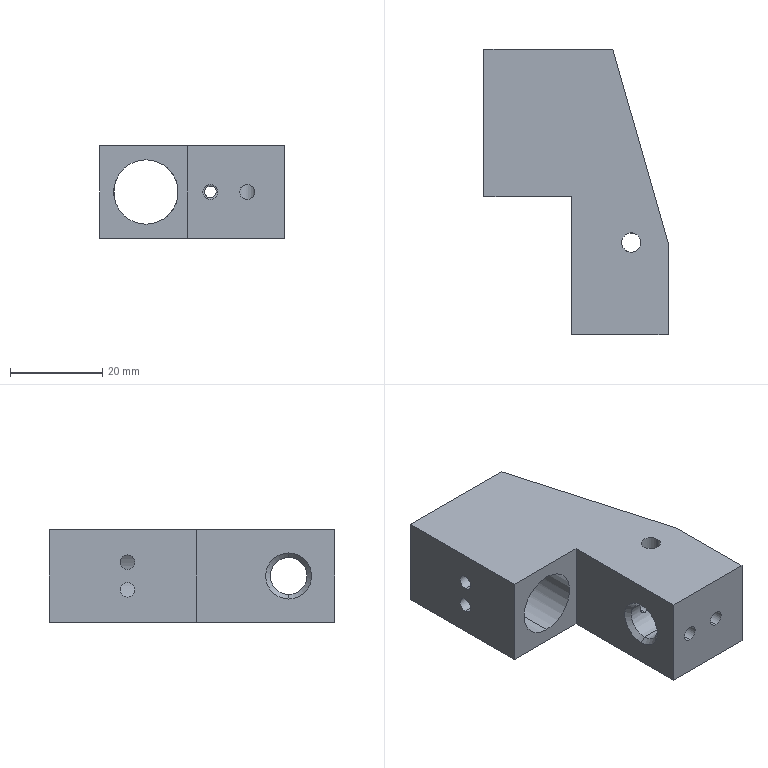Part | SolidWorks | features ICE 6, HoleWzd 4, 3DProfileFeature 3, Chamfer 2, Extrusion 1, LPattern 1, RefAxis 1 | 1 solid | 54 faces | box 40 x 62 x 20 mm | volume 25911 mm3 | cylinder 28 | cone 14 | plane 12 | commonest cylinder face diameters 2.5 x10 3.3 x6 3.2 x4 4 x2 4.2 x2 8 x2